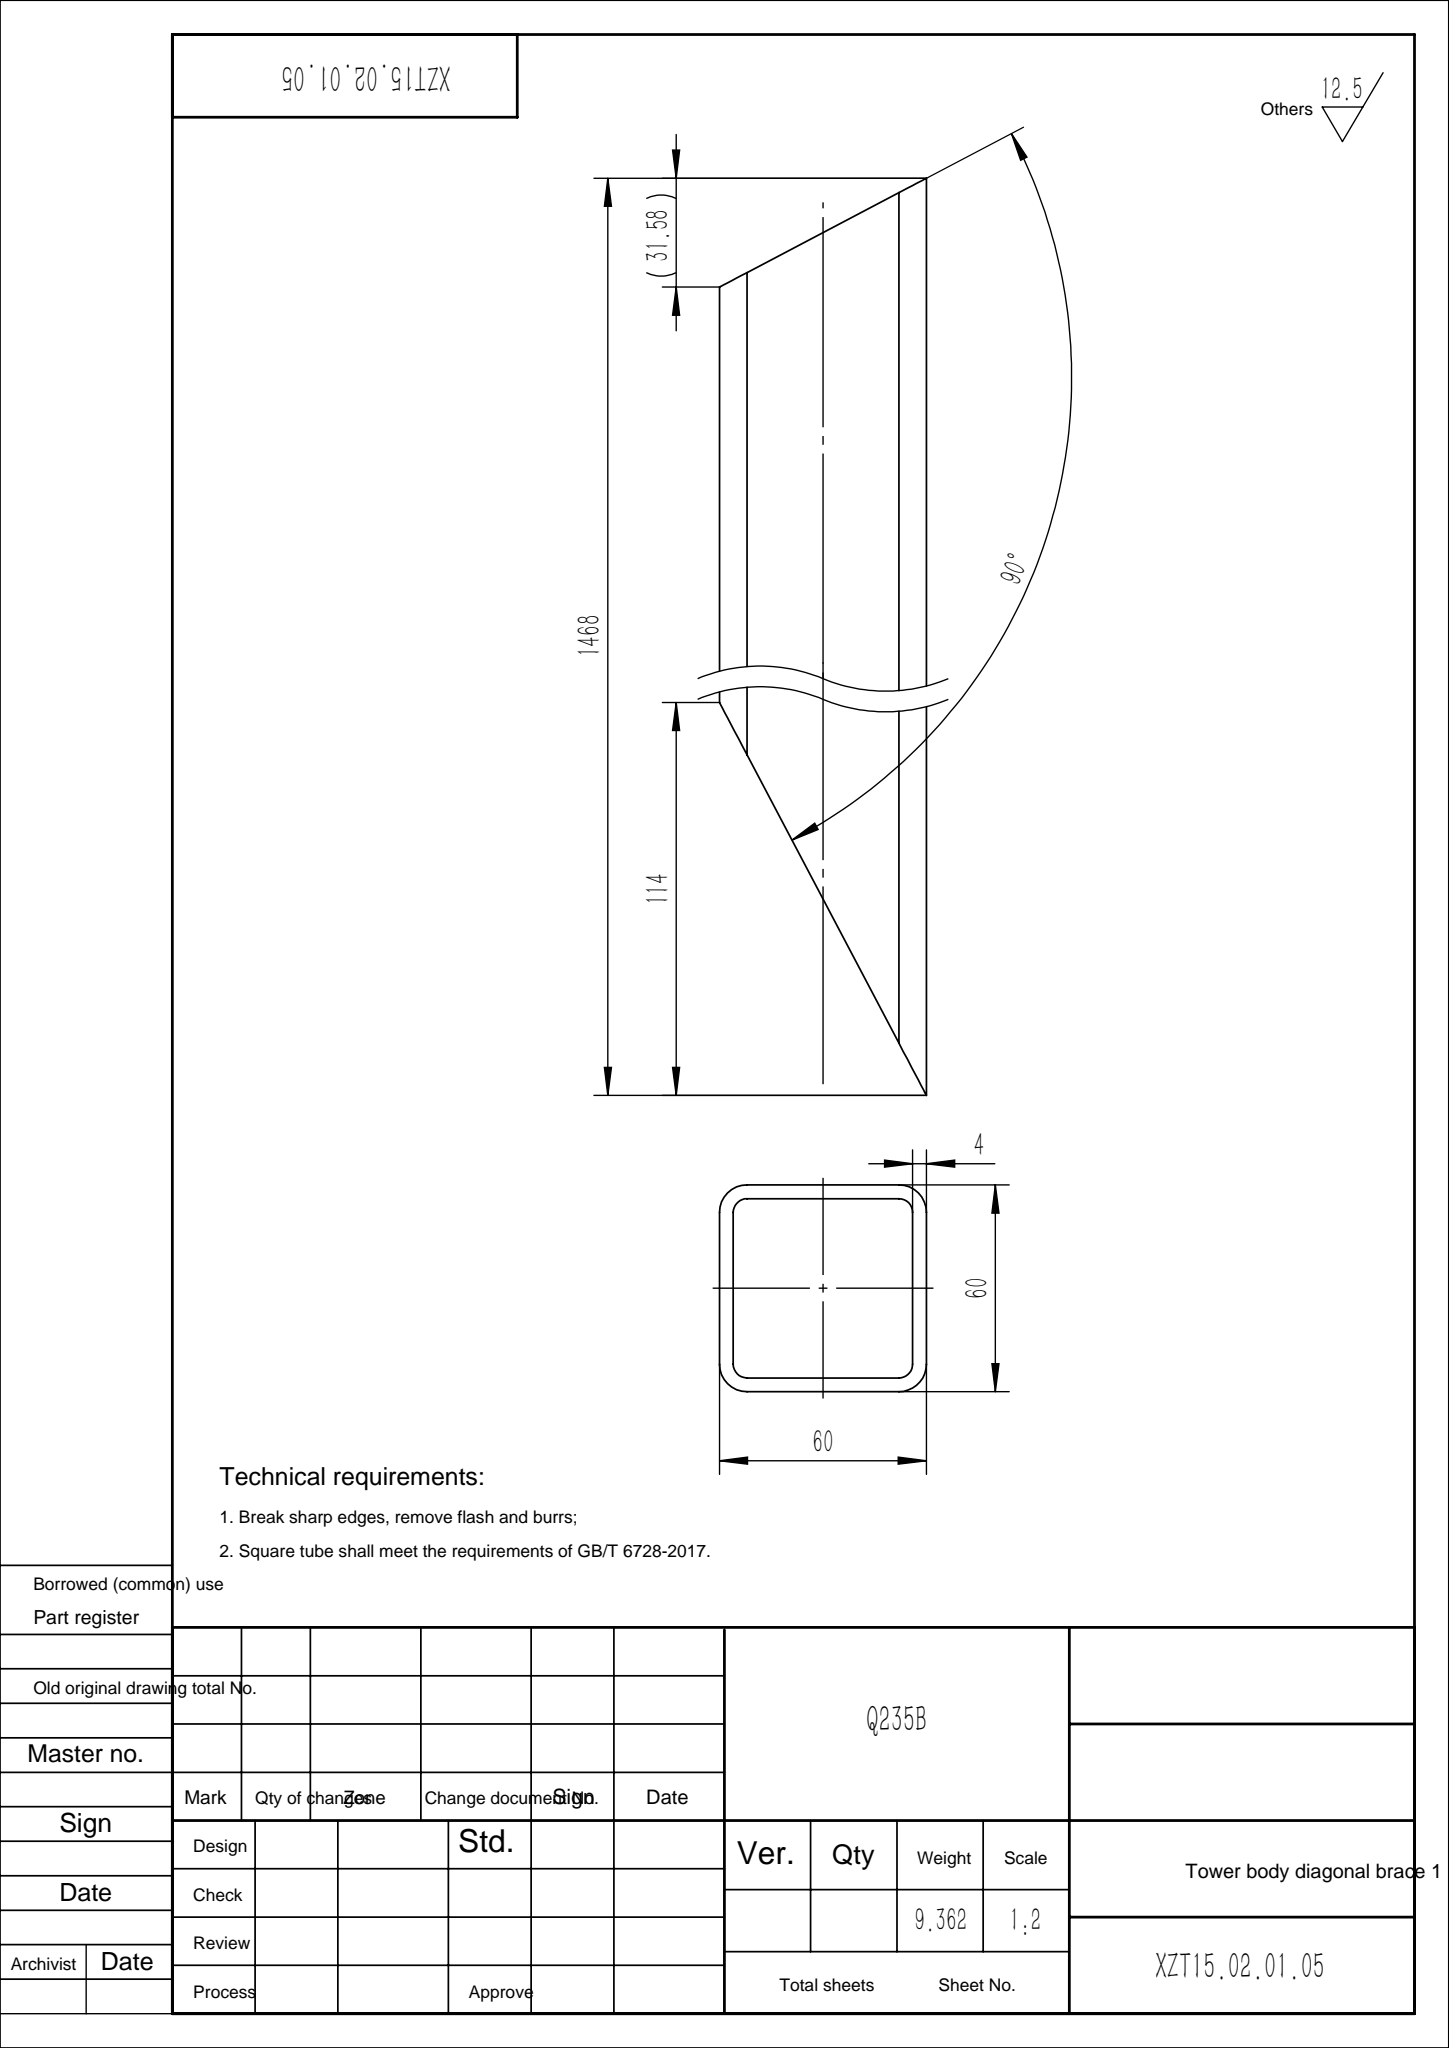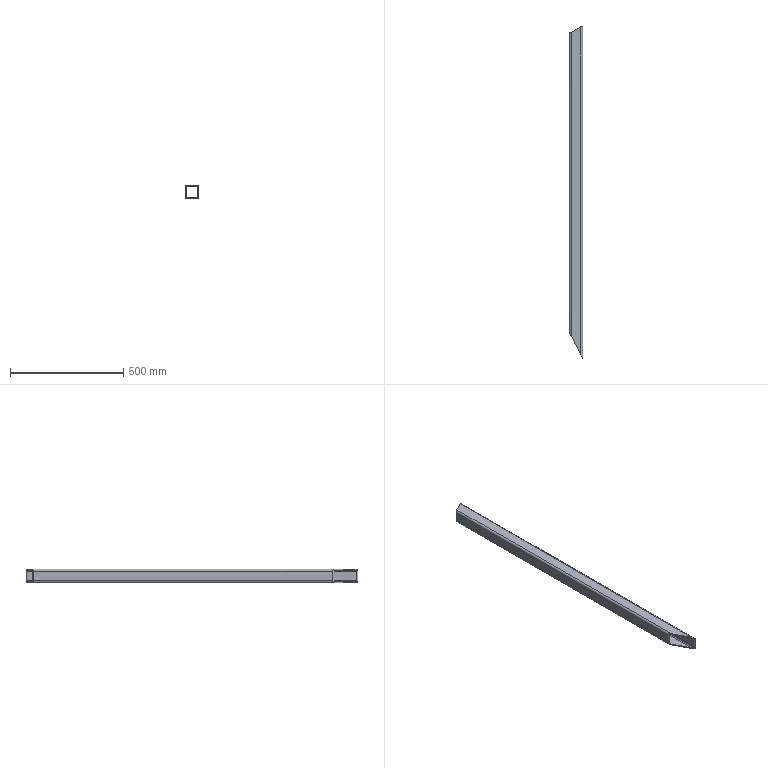Part | SolidWorks | features ICE 1, WeldMemberFeat 1, WeldmentFeature 1 | 1 solid | 18 faces | box 60 x 1468 x 60 mm | volume 1192621 mm3 | plane 10 | cylinder 8 | commonest cylinder face diameters 8 x4 16 x4
STEP:
#1=CARTESIAN_POINT('',(30.,0.,22.));
#2=VERTEX_POINT('',#1);
#3=CARTESIAN_POINT('',(30.,0.,-22.));
#4=VERTEX_POINT('',#3);
#5=CARTESIAN_POINT('',(30.,0.,-22.));
#6=DIRECTION('',(0.,0.,-1.));
#7=VECTOR('',#6,1000.);
#8=LINE('',#5,#7);
#9=EDGE_CURVE('',#2,#4,#8,.T.);
#10=ORIENTED_EDGE('',*,*,#9,.T.);
#11=CARTESIAN_POINT('',(30.,1468.,-22.));
#12=VERTEX_POINT('',#11);
#13=CARTESIAN_POINT('',(30.,1468.,-22.));
#14=DIRECTION('',(0.,-1.,0.));
#15=VECTOR('',#14,1000.);
#16=LINE('',#13,#15);
#17=EDGE_CURVE('',#12,#4,#16,.T.);
#18=ORIENTED_EDGE('',*,*,#17,.F.);
#19=CARTESIAN_POINT('',(30.,1468.,22.));
#20=VERTEX_POINT('',#19);
#21=CARTESIAN_POINT('',(30.,1468.,-22.));
#22=DIRECTION('',(0.,0.,-1.));
#23=VECTOR('',#22,1000.);
#24=LINE('',#21,#23);
#25=EDGE_CURVE('',#20,#12,#24,.T.);
#26=ORIENTED_EDGE('',*,*,#25,.F.);
#27=CARTESIAN_POINT('',(30.,1468.,22.));
#28=DIRECTION('',(0.,-1.,0.));
#29=VECTOR('',#28,1000.);
#30=LINE('',#27,#29);
#31=EDGE_CURVE('',#20,#2,#30,.T.);
#32=ORIENTED_EDGE('',*,*,#31,.T.);
#33=EDGE_LOOP('',(#10,#18,#26,#32));
#34=FACE_OUTER_BOUND('',#33,.T.);
#35=CARTESIAN_POINT('',(30.,1468.,-22.));
#36=DIRECTION('',(-1.,0.,0.));
#37=DIRECTION('',(0.,0.,1.));
#38=AXIS2_PLACEMENT_3D('',#35,#36,#37);
#39=PLANE('',#38);
#40=ADVANCED_FACE('',(#34),#39,.F.);
#41=CARTESIAN_POINT('',(-30.,1436.421,22.));
#42=VERTEX_POINT('',#41);
#43=CARTESIAN_POINT('',(-30.,114.,22.));
#44=VERTEX_POINT('',#43);
#45=CARTESIAN_POINT('',(-30.,1468.,22.));
#46=DIRECTION('',(0.,-1.,0.));
#47=VECTOR('',#46,1000.);
#48=LINE('',#45,#47);
#49=EDGE_CURVE('',#42,#44,#48,.T.);
#50=ORIENTED_EDGE('',*,*,#49,.F.);
#51=CARTESIAN_POINT('',(-30.,1436.421,-22.));
#52=VERTEX_POINT('',#51);
#53=CARTESIAN_POINT('',(-30.,1436.421,-30.));
#54=DIRECTION('',(0.,0.,1.));
#55=VECTOR('',#54,1000.);
#56=LINE('',#53,#55);
#57=EDGE_CURVE('',#52,#42,#56,.T.);
#58=ORIENTED_EDGE('',*,*,#57,.F.);
#59=CARTESIAN_POINT('',(-30.,114.,-22.));
#60=VERTEX_POINT('',#59);
#61=CARTESIAN_POINT('',(-30.,1468.,-22.));
#62=DIRECTION('',(0.,-1.,0.));
#63=VECTOR('',#62,1000.);
#64=LINE('',#61,#63);
#65=EDGE_CURVE('',#52,#60,#64,.T.);
#66=ORIENTED_EDGE('',*,*,#65,.T.);
#67=CARTESIAN_POINT('',(-30.,114.,-30.));
#68=DIRECTION('',(0.,0.,1.));
#69=VECTOR('',#68,1000.);
#70=LINE('',#67,#69);
#71=EDGE_CURVE('',#60,#44,#70,.T.);
#72=ORIENTED_EDGE('',*,*,#71,.T.);
#73=EDGE_LOOP('',(#50,#58,#66,#72));
#74=FACE_OUTER_BOUND('',#73,.T.);
#75=CARTESIAN_POINT('',(-30.,1468.,22.));
#76=DIRECTION('',(1.,0.,0.));
#77=DIRECTION('',(0.,0.,-1.));
#78=AXIS2_PLACEMENT_3D('',#75,#76,#77);
#79=PLANE('',#78);
#80=ADVANCED_FACE('',(#74),#79,.F.);
#81=ORIENTED_EDGE('',*,*,#65,.F.);
#82=CARTESIAN_POINT('',(-22.,1440.632,-30.));
#83=VERTEX_POINT('',#82);
#84=CARTESIAN_POINT('',(-30.,1436.421,-22.));
#85=CARTESIAN_POINT('',(-30.,1436.421,-26.686));
#86=CARTESIAN_POINT('',(-26.686,1438.165,-30.));
#87=CARTESIAN_POINT('',(-22.,1440.632,-30.));
#88=(BOUNDED_CURVE()B_SPLINE_CURVE(3,(#84,#85,#86,#87),.UNSPECIFIED.,.F.,.F.)B_SPLINE_CURVE_WITH_KNOTS((4,4),(0.,1.571),.UNSPECIFIED.)CURVE()GEOMETRIC_REPRESENTATION_ITEM()RATIONAL_B_SPLINE_CURVE((1.,0.8047,0.8047,1.))REPRESENTATION_ITEM(''));
#89=EDGE_CURVE('',#52,#83,#88,.T.);
#90=ORIENTED_EDGE('',*,*,#89,.T.);
#91=CARTESIAN_POINT('',(-22.,98.8,-30.));
#92=VERTEX_POINT('',#91);
#93=CARTESIAN_POINT('',(-22.,1468.,-30.));
#94=DIRECTION('',(0.,-1.,0.));
#95=VECTOR('',#94,1000.);
#96=LINE('',#93,#95);
#97=EDGE_CURVE('',#83,#92,#96,.T.);
#98=ORIENTED_EDGE('',*,*,#97,.T.);
#99=CARTESIAN_POINT('',(-22.,98.8,-30.));
#100=CARTESIAN_POINT('',(-26.686,107.704,-30.));
#101=CARTESIAN_POINT('',(-30.,114.,-26.686));
#102=CARTESIAN_POINT('',(-30.,114.,-22.));
#103=(BOUNDED_CURVE()B_SPLINE_CURVE(3,(#99,#100,#101,#102),.UNSPECIFIED.,.F.,.F.)B_SPLINE_CURVE_WITH_KNOTS((4,4),(1.571,3.142),.UNSPECIFIED.)CURVE()GEOMETRIC_REPRESENTATION_ITEM()RATIONAL_B_SPLINE_CURVE((1.,0.8047,0.8047,1.))REPRESENTATION_ITEM(''));
#104=EDGE_CURVE('',#92,#60,#103,.T.);
#105=ORIENTED_EDGE('',*,*,#104,.T.);
#106=EDGE_LOOP('',(#81,#90,#98,#105));
#107=FACE_OUTER_BOUND('',#106,.T.);
#108=CARTESIAN_POINT('',(-22.,1468.,-22.));
#109=DIRECTION('',(0.,-1.,0.));
#110=DIRECTION('',(0.,0.,-1.));
#111=AXIS2_PLACEMENT_3D('',#108,#109,#110);
#112=CYLINDRICAL_SURFACE('',#111,8.);
#113=ADVANCED_FACE('',(#107),#112,.T.);
#114=ORIENTED_EDGE('',*,*,#97,.F.);
#115=CARTESIAN_POINT('',(22.,1463.789,-30.));
#116=VERTEX_POINT('',#115);
#117=CARTESIAN_POINT('',(-30.,1436.421,-30.));
#118=DIRECTION('',(0.8849,0.4657,0.));
#119=VECTOR('',#118,1000.);
#120=LINE('',#117,#119);
#121=EDGE_CURVE('',#83,#116,#120,.T.);
#122=ORIENTED_EDGE('',*,*,#121,.T.);
#123=CARTESIAN_POINT('',(22.,15.2,-30.));
#124=VERTEX_POINT('',#123);
#125=CARTESIAN_POINT('',(22.,1468.,-30.));
#126=DIRECTION('',(0.,-1.,0.));
#127=VECTOR('',#126,1000.);
#128=LINE('',#125,#127);
#129=EDGE_CURVE('',#116,#124,#128,.T.);
#130=ORIENTED_EDGE('',*,*,#129,.T.);
#131=CARTESIAN_POINT('',(-30.,114.,-30.));
#132=DIRECTION('',(-0.4657,0.8849,0.));
#133=VECTOR('',#132,1000.);
#134=LINE('',#131,#133);
#135=EDGE_CURVE('',#124,#92,#134,.T.);
#136=ORIENTED_EDGE('',*,*,#135,.T.);
#137=EDGE_LOOP('',(#114,#122,#130,#136));
#138=FACE_OUTER_BOUND('',#137,.T.);
#139=CARTESIAN_POINT('',(22.,1468.,-30.));
#140=DIRECTION('',(0.,0.,1.));
#141=DIRECTION('',(1.,0.,0.));
#142=AXIS2_PLACEMENT_3D('',#139,#140,#141);
#143=PLANE('',#142);
#144=ADVANCED_FACE('',(#138),#143,.F.);
#145=ORIENTED_EDGE('',*,*,#129,.F.);
#146=CARTESIAN_POINT('',(22.,1463.789,-30.));
#147=CARTESIAN_POINT('',(26.686,1466.256,-30.));
#148=CARTESIAN_POINT('',(30.,1468.,-26.686));
#149=CARTESIAN_POINT('',(30.,1468.,-22.));
#150=(BOUNDED_CURVE()B_SPLINE_CURVE(3,(#146,#147,#148,#149),.UNSPECIFIED.,.F.,.T.)B_SPLINE_CURVE_WITH_KNOTS((4,4),(1.571,3.142),.UNSPECIFIED.)CURVE()GEOMETRIC_REPRESENTATION_ITEM()RATIONAL_B_SPLINE_CURVE((1.,0.8047,0.8047,1.))REPRESENTATION_ITEM(''));
#151=EDGE_CURVE('',#116,#12,#150,.T.);
#152=ORIENTED_EDGE('',*,*,#151,.T.);
#153=ORIENTED_EDGE('',*,*,#17,.T.);
#154=CARTESIAN_POINT('',(30.,0.,-22.));
#155=CARTESIAN_POINT('',(30.,0.,-26.686));
#156=CARTESIAN_POINT('',(26.686,6.296,-30.));
#157=CARTESIAN_POINT('',(22.,15.2,-30.));
#158=(BOUNDED_CURVE()B_SPLINE_CURVE(3,(#154,#155,#156,#157),.UNSPECIFIED.,.F.,.F.)B_SPLINE_CURVE_WITH_KNOTS((4,4),(0.,1.571),.UNSPECIFIED.)CURVE()GEOMETRIC_REPRESENTATION_ITEM()RATIONAL_B_SPLINE_CURVE((1.,0.8047,0.8047,1.))REPRESENTATION_ITEM(''));
#159=EDGE_CURVE('',#4,#124,#158,.T.);
#160=ORIENTED_EDGE('',*,*,#159,.T.);
#161=EDGE_LOOP('',(#145,#152,#153,#160));
#162=FACE_OUTER_BOUND('',#161,.T.);
#163=CARTESIAN_POINT('',(22.,1468.,-22.));
#164=DIRECTION('',(0.,-1.,0.));
#165=DIRECTION('',(0.,0.,-1.));
#166=AXIS2_PLACEMENT_3D('',#163,#164,#165);
#167=CYLINDRICAL_SURFACE('',#166,8.);
#168=ADVANCED_FACE('',(#162),#167,.T.);
#169=ORIENTED_EDGE('',*,*,#31,.F.);
#170=CARTESIAN_POINT('',(22.,1463.789,30.));
#171=VERTEX_POINT('',#170);
#172=CARTESIAN_POINT('',(30.,1468.,22.));
#173=CARTESIAN_POINT('',(30.,1468.,26.686));
#174=CARTESIAN_POINT('',(26.686,1466.256,30.));
#175=CARTESIAN_POINT('',(22.,1463.789,30.));
#176=(BOUNDED_CURVE()B_SPLINE_CURVE(3,(#172,#173,#174,#175),.UNSPECIFIED.,.F.,.F.)B_SPLINE_CURVE_WITH_KNOTS((4,4),(3.142,4.712),.UNSPECIFIED.)CURVE()GEOMETRIC_REPRESENTATION_ITEM()RATIONAL_B_SPLINE_CURVE((1.,0.8047,0.8047,1.))REPRESENTATION_ITEM(''));
#177=EDGE_CURVE('',#20,#171,#176,.T.);
#178=ORIENTED_EDGE('',*,*,#177,.T.);
#179=CARTESIAN_POINT('',(22.,15.2,30.));
#180=VERTEX_POINT('',#179);
#181=CARTESIAN_POINT('',(22.,1468.,30.));
#182=DIRECTION('',(0.,-1.,0.));
#183=VECTOR('',#182,1000.);
#184=LINE('',#181,#183);
#185=EDGE_CURVE('',#171,#180,#184,.T.);
#186=ORIENTED_EDGE('',*,*,#185,.T.);
#187=CARTESIAN_POINT('',(22.,15.2,30.));
#188=CARTESIAN_POINT('',(26.686,6.296,30.));
#189=CARTESIAN_POINT('',(30.,0.,26.686));
#190=CARTESIAN_POINT('',(30.,0.,22.));
#191=(BOUNDED_CURVE()B_SPLINE_CURVE(3,(#187,#188,#189,#190),.UNSPECIFIED.,.F.,.F.)B_SPLINE_CURVE_WITH_KNOTS((4,4),(4.712,6.283),.UNSPECIFIED.)CURVE()GEOMETRIC_REPRESENTATION_ITEM()RATIONAL_B_SPLINE_CURVE((1.,0.8047,0.8047,1.))REPRESENTATION_ITEM(''));
#192=EDGE_CURVE('',#180,#2,#191,.T.);
#193=ORIENTED_EDGE('',*,*,#192,.T.);
#194=EDGE_LOOP('',(#169,#178,#186,#193));
#195=FACE_OUTER_BOUND('',#194,.T.);
#196=CARTESIAN_POINT('',(22.,1468.,22.));
#197=DIRECTION('',(0.,-1.,0.));
#198=DIRECTION('',(0.,0.,-1.));
#199=AXIS2_PLACEMENT_3D('',#196,#197,#198);
#200=CYLINDRICAL_SURFACE('',#199,8.);
#201=ADVANCED_FACE('',(#195),#200,.T.);
#202=ORIENTED_EDGE('',*,*,#185,.F.);
#203=CARTESIAN_POINT('',(-22.,1440.632,30.));
#204=VERTEX_POINT('',#203);
#205=CARTESIAN_POINT('',(-10.72,1446.568,30.));
#206=DIRECTION('',(-0.8849,-0.4657,0.));
#207=VECTOR('',#206,1000.);
#208=LINE('',#205,#207);
#209=EDGE_CURVE('',#171,#204,#208,.T.);
#210=ORIENTED_EDGE('',*,*,#209,.T.);
#211=CARTESIAN_POINT('',(-22.,98.8,30.));
#212=VERTEX_POINT('',#211);
#213=CARTESIAN_POINT('',(-22.,1468.,30.));
#214=DIRECTION('',(0.,-1.,0.));
#215=VECTOR('',#214,1000.);
#216=LINE('',#213,#215);
#217=EDGE_CURVE('',#204,#212,#216,.T.);
#218=ORIENTED_EDGE('',*,*,#217,.T.);
#219=CARTESIAN_POINT('',(-586.312,1170.993,30.));
#220=DIRECTION('',(0.4657,-0.8849,0.));
#221=VECTOR('',#220,1000.);
#222=LINE('',#219,#221);
#223=EDGE_CURVE('',#212,#180,#222,.T.);
#224=ORIENTED_EDGE('',*,*,#223,.T.);
#225=EDGE_LOOP('',(#202,#210,#218,#224));
#226=FACE_OUTER_BOUND('',#225,.T.);
#227=CARTESIAN_POINT('',(-22.,1468.,30.));
#228=DIRECTION('',(0.,0.,-1.));
#229=DIRECTION('',(-1.,0.,0.));
#230=AXIS2_PLACEMENT_3D('',#227,#228,#229);
#231=PLANE('',#230);
#232=ADVANCED_FACE('',(#226),#231,.F.);
#233=ORIENTED_EDGE('',*,*,#217,.F.);
#234=CARTESIAN_POINT('',(-22.,1440.632,30.));
#235=CARTESIAN_POINT('',(-26.686,1438.165,30.));
#236=CARTESIAN_POINT('',(-30.,1436.421,26.686));
#237=CARTESIAN_POINT('',(-30.,1436.421,22.));
#238=(BOUNDED_CURVE()B_SPLINE_CURVE(3,(#234,#235,#236,#237),.UNSPECIFIED.,.F.,.F.)B_SPLINE_CURVE_WITH_KNOTS((4,4),(4.712,6.283),.UNSPECIFIED.)CURVE()GEOMETRIC_REPRESENTATION_ITEM()RATIONAL_B_SPLINE_CURVE((1.,0.8047,0.8047,1.))REPRESENTATION_ITEM(''));
#239=EDGE_CURVE('',#204,#42,#238,.T.);
#240=ORIENTED_EDGE('',*,*,#239,.T.);
#241=ORIENTED_EDGE('',*,*,#49,.T.);
#242=CARTESIAN_POINT('',(-30.,114.,22.));
#243=CARTESIAN_POINT('',(-30.,114.,26.686));
#244=CARTESIAN_POINT('',(-26.686,107.704,30.));
#245=CARTESIAN_POINT('',(-22.,98.8,30.));
#246=(BOUNDED_CURVE()B_SPLINE_CURVE(3,(#242,#243,#244,#245),.UNSPECIFIED.,.F.,.F.)B_SPLINE_CURVE_WITH_KNOTS((4,4),(3.142,4.712),.UNSPECIFIED.)CURVE()GEOMETRIC_REPRESENTATION_ITEM()RATIONAL_B_SPLINE_CURVE((1.,0.8047,0.8047,1.))REPRESENTATION_ITEM(''));
#247=EDGE_CURVE('',#44,#212,#246,.T.);
#248=ORIENTED_EDGE('',*,*,#247,.T.);
#249=EDGE_LOOP('',(#233,#240,#241,#248));
#250=FACE_OUTER_BOUND('',#249,.T.);
#251=CARTESIAN_POINT('',(-22.,1468.,22.));
#252=DIRECTION('',(0.,-1.,0.));
#253=DIRECTION('',(0.,0.,-1.));
#254=AXIS2_PLACEMENT_3D('',#251,#252,#253);
#255=CYLINDRICAL_SURFACE('',#254,8.);
#256=ADVANCED_FACE('',(#250),#255,.T.);
#257=CARTESIAN_POINT('',(22.,15.2,26.));
#258=VERTEX_POINT('',#257);
#259=CARTESIAN_POINT('',(26.,7.6,22.));
#260=VERTEX_POINT('',#259);
#261=CARTESIAN_POINT('',(22.,15.2,26.));
#262=CARTESIAN_POINT('',(24.343,10.748,26.));
#263=CARTESIAN_POINT('',(26.,7.6,24.343));
#264=CARTESIAN_POINT('',(26.,7.6,22.));
#265=(BOUNDED_CURVE()B_SPLINE_CURVE(3,(#261,#262,#263,#264),.UNSPECIFIED.,.F.,.F.)B_SPLINE_CURVE_WITH_KNOTS((4,4),(4.712,6.283),.UNSPECIFIED.)CURVE()GEOMETRIC_REPRESENTATION_ITEM()RATIONAL_B_SPLINE_CURVE((1.,0.8047,0.8047,1.))REPRESENTATION_ITEM(''));
#266=EDGE_CURVE('',#258,#260,#265,.T.);
#267=ORIENTED_EDGE('',*,*,#266,.T.);
#268=CARTESIAN_POINT('',(26.,7.6,-22.));
#269=VERTEX_POINT('',#268);
#270=CARTESIAN_POINT('',(26.,7.6,-22.));
#271=DIRECTION('',(0.,0.,-1.));
#272=VECTOR('',#271,1000.);
#273=LINE('',#270,#272);
#274=EDGE_CURVE('',#260,#269,#273,.T.);
#275=ORIENTED_EDGE('',*,*,#274,.T.);
#276=CARTESIAN_POINT('',(22.,15.2,-26.));
#277=VERTEX_POINT('',#276);
#278=CARTESIAN_POINT('',(26.,7.6,-22.));
#279=CARTESIAN_POINT('',(26.,7.6,-24.343));
#280=CARTESIAN_POINT('',(24.343,10.748,-26.));
#281=CARTESIAN_POINT('',(22.,15.2,-26.));
#282=(BOUNDED_CURVE()B_SPLINE_CURVE(3,(#278,#279,#280,#281),.UNSPECIFIED.,.F.,.F.)B_SPLINE_CURVE_WITH_KNOTS((4,4),(0.,1.571),.UNSPECIFIED.)CURVE()GEOMETRIC_REPRESENTATION_ITEM()RATIONAL_B_SPLINE_CURVE((1.,0.8047,0.8047,1.))REPRESENTATION_ITEM(''));
#283=EDGE_CURVE('',#269,#277,#282,.T.);
#284=ORIENTED_EDGE('',*,*,#283,.T.);
#285=CARTESIAN_POINT('',(-22.,98.8,-26.));
#286=VERTEX_POINT('',#285);
#287=CARTESIAN_POINT('',(-576.768,1152.859,-26.));
#288=DIRECTION('',(-0.4657,0.8849,0.));
#289=VECTOR('',#288,1000.);
#290=LINE('',#287,#289);
#291=EDGE_CURVE('',#277,#286,#290,.T.);
#292=ORIENTED_EDGE('',*,*,#291,.T.);
#293=CARTESIAN_POINT('',(-26.,106.4,-22.));
#294=VERTEX_POINT('',#293);
#295=CARTESIAN_POINT('',(-22.,98.8,-26.));
#296=CARTESIAN_POINT('',(-24.343,103.252,-26.));
#297=CARTESIAN_POINT('',(-26.,106.4,-24.343));
#298=CARTESIAN_POINT('',(-26.,106.4,-22.));
#299=(BOUNDED_CURVE()B_SPLINE_CURVE(3,(#295,#296,#297,#298),.UNSPECIFIED.,.F.,.T.)B_SPLINE_CURVE_WITH_KNOTS((4,4),(1.571,3.142),.UNSPECIFIED.)CURVE()GEOMETRIC_REPRESENTATION_ITEM()RATIONAL_B_SPLINE_CURVE((1.,0.8047,0.8047,1.))REPRESENTATION_ITEM(''));
#300=EDGE_CURVE('',#286,#294,#299,.T.);
#301=ORIENTED_EDGE('',*,*,#300,.T.);
#302=CARTESIAN_POINT('',(-26.,106.4,22.));
#303=VERTEX_POINT('',#302);
#304=CARTESIAN_POINT('',(-26.,106.4,22.));
#305=DIRECTION('',(0.,0.,1.));
#306=VECTOR('',#305,1000.);
#307=LINE('',#304,#306);
#308=EDGE_CURVE('',#294,#303,#307,.T.);
#309=ORIENTED_EDGE('',*,*,#308,.T.);
#310=CARTESIAN_POINT('',(-22.,98.8,26.));
#311=VERTEX_POINT('',#310);
#312=CARTESIAN_POINT('',(-26.,106.4,22.));
#313=CARTESIAN_POINT('',(-26.,106.4,24.343));
#314=CARTESIAN_POINT('',(-24.343,103.252,26.));
#315=CARTESIAN_POINT('',(-22.,98.8,26.));
#316=(BOUNDED_CURVE()B_SPLINE_CURVE(3,(#312,#313,#314,#315),.UNSPECIFIED.,.F.,.F.)B_SPLINE_CURVE_WITH_KNOTS((4,4),(3.142,4.712),.UNSPECIFIED.)CURVE()GEOMETRIC_REPRESENTATION_ITEM()RATIONAL_B_SPLINE_CURVE((1.,0.8047,0.8047,1.))REPRESENTATION_ITEM(''));
#317=EDGE_CURVE('',#303,#311,#316,.T.);
#318=ORIENTED_EDGE('',*,*,#317,.T.);
#319=CARTESIAN_POINT('',(-586.312,1170.993,26.));
#320=DIRECTION('',(0.4657,-0.8849,0.));
#321=VECTOR('',#320,1000.);
#322=LINE('',#319,#321);
#323=EDGE_CURVE('',#311,#258,#322,.T.);
#324=ORIENTED_EDGE('',*,*,#323,.T.);
#325=EDGE_LOOP('',(#267,#275,#284,#292,#301,#309,#318,#324));
#326=FACE_BOUND('',#325,.T.);
#327=ORIENTED_EDGE('',*,*,#71,.F.);
#328=ORIENTED_EDGE('',*,*,#104,.F.);
#329=ORIENTED_EDGE('',*,*,#135,.F.);
#330=ORIENTED_EDGE('',*,*,#159,.F.);
#331=ORIENTED_EDGE('',*,*,#9,.F.);
#332=ORIENTED_EDGE('',*,*,#192,.F.);
#333=ORIENTED_EDGE('',*,*,#223,.F.);
#334=ORIENTED_EDGE('',*,*,#247,.F.);
#335=EDGE_LOOP('',(#327,#328,#329,#330,#331,#332,#333,#334));
#336=FACE_OUTER_BOUND('',#335,.T.);
#337=CARTESIAN_POINT('',(-30.,114.,-30.));
#338=DIRECTION('',(0.8849,0.4657,0.));
#339=DIRECTION('',(-0.4657,0.8849,0.));
#340=AXIS2_PLACEMENT_3D('',#337,#338,#339);
#341=PLANE('',#340);
#342=ADVANCED_FACE('',(#326,#336),#341,.F.);
#343=CARTESIAN_POINT('',(26.,1465.895,22.));
#344=VERTEX_POINT('',#343);
#345=CARTESIAN_POINT('',(22.,1463.789,26.));
#346=VERTEX_POINT('',#345);
#347=CARTESIAN_POINT('',(26.,1465.895,22.));
#348=CARTESIAN_POINT('',(26.,1465.895,24.343));
#349=CARTESIAN_POINT('',(24.343,1465.023,26.));
#350=CARTESIAN_POINT('',(22.,1463.789,26.));
#351=(BOUNDED_CURVE()B_SPLINE_CURVE(3,(#347,#348,#349,#350),.UNSPECIFIED.,.F.,.F.)B_SPLINE_CURVE_WITH_KNOTS((4,4),(3.142,4.712),.UNSPECIFIED.)CURVE()GEOMETRIC_REPRESENTATION_ITEM()RATIONAL_B_SPLINE_CURVE((1.,0.8047,0.8047,1.))REPRESENTATION_ITEM(''));
#352=EDGE_CURVE('',#344,#346,#351,.T.);
#353=ORIENTED_EDGE('',*,*,#352,.T.);
#354=CARTESIAN_POINT('',(-22.,1440.632,26.));
#355=VERTEX_POINT('',#354);
#356=CARTESIAN_POINT('',(-10.72,1446.568,26.));
#357=DIRECTION('',(-0.8849,-0.4657,0.));
#358=VECTOR('',#357,1000.);
#359=LINE('',#356,#358);
#360=EDGE_CURVE('',#346,#355,#359,.T.);
#361=ORIENTED_EDGE('',*,*,#360,.T.);
#362=CARTESIAN_POINT('',(-26.,1438.526,22.));
#363=VERTEX_POINT('',#362);
#364=CARTESIAN_POINT('',(-22.,1440.632,26.));
#365=CARTESIAN_POINT('',(-24.343,1439.398,26.));
#366=CARTESIAN_POINT('',(-26.,1438.526,24.343));
#367=CARTESIAN_POINT('',(-26.,1438.526,22.));
#368=(BOUNDED_CURVE()B_SPLINE_CURVE(3,(#364,#365,#366,#367),.UNSPECIFIED.,.F.,.F.)B_SPLINE_CURVE_WITH_KNOTS((4,4),(4.712,6.283),.UNSPECIFIED.)CURVE()GEOMETRIC_REPRESENTATION_ITEM()RATIONAL_B_SPLINE_CURVE((1.,0.8047,0.8047,1.))REPRESENTATION_ITEM(''));
#369=EDGE_CURVE('',#355,#363,#368,.T.);
#370=ORIENTED_EDGE('',*,*,#369,.T.);
#371=CARTESIAN_POINT('',(-26.,1438.526,-22.));
#372=VERTEX_POINT('',#371);
#373=CARTESIAN_POINT('',(-26.,1438.526,22.));
#374=DIRECTION('',(0.,0.,-1.));
#375=VECTOR('',#374,1000.);
#376=LINE('',#373,#375);
#377=EDGE_CURVE('',#363,#372,#376,.T.);
#378=ORIENTED_EDGE('',*,*,#377,.T.);
#379=CARTESIAN_POINT('',(-22.,1440.632,-26.));
#380=VERTEX_POINT('',#379);
#381=CARTESIAN_POINT('',(-26.,1438.526,-22.));
#382=CARTESIAN_POINT('',(-26.,1438.526,-24.343));
#383=CARTESIAN_POINT('',(-24.343,1439.398,-26.));
#384=CARTESIAN_POINT('',(-22.,1440.632,-26.));
#385=(BOUNDED_CURVE()B_SPLINE_CURVE(3,(#381,#382,#383,#384),.UNSPECIFIED.,.F.,.F.)B_SPLINE_CURVE_WITH_KNOTS((4,4),(0.,1.571),.UNSPECIFIED.)CURVE()GEOMETRIC_REPRESENTATION_ITEM()RATIONAL_B_SPLINE_CURVE((1.,0.8047,0.8047,1.))REPRESENTATION_ITEM(''));
#386=EDGE_CURVE('',#372,#380,#385,.T.);
#387=ORIENTED_EDGE('',*,*,#386,.T.);
#388=CARTESIAN_POINT('',(22.,1463.789,-26.));
#389=VERTEX_POINT('',#388);
#390=CARTESIAN_POINT('',(23.735,1464.703,-26.));
#391=DIRECTION('',(0.8849,0.4657,0.));
#392=VECTOR('',#391,1000.);
#393=LINE('',#390,#392);
#394=EDGE_CURVE('',#380,#389,#393,.T.);
#395=ORIENTED_EDGE('',*,*,#394,.T.);
#396=CARTESIAN_POINT('',(26.,1465.895,-22.));
#397=VERTEX_POINT('',#396);
#398=CARTESIAN_POINT('',(22.,1463.789,-26.));
#399=CARTESIAN_POINT('',(24.343,1465.023,-26.));
#400=CARTESIAN_POINT('',(26.,1465.895,-24.343));
#401=CARTESIAN_POINT('',(26.,1465.895,-22.));
#402=(BOUNDED_CURVE()B_SPLINE_CURVE(3,(#398,#399,#400,#401),.UNSPECIFIED.,.F.,.F.)B_SPLINE_CURVE_WITH_KNOTS((4,4),(1.571,3.142),.UNSPECIFIED.)CURVE()GEOMETRIC_REPRESENTATION_ITEM()RATIONAL_B_SPLINE_CURVE((1.,0.8047,0.8047,1.))REPRESENTATION_ITEM(''));
#403=EDGE_CURVE('',#389,#397,#402,.T.);
#404=ORIENTED_EDGE('',*,*,#403,.T.);
#405=CARTESIAN_POINT('',(26.,1465.895,-22.));
#406=DIRECTION('',(0.,0.,1.));
#407=VECTOR('',#406,1000.);
#408=LINE('',#405,#407);
#409=EDGE_CURVE('',#397,#344,#408,.T.);
#410=ORIENTED_EDGE('',*,*,#409,.T.);
#411=EDGE_LOOP('',(#353,#361,#370,#378,#387,#395,#404,#410));
#412=FACE_BOUND('',#411,.T.);
#413=ORIENTED_EDGE('',*,*,#209,.F.);
#414=ORIENTED_EDGE('',*,*,#177,.F.);
#415=ORIENTED_EDGE('',*,*,#25,.T.);
#416=ORIENTED_EDGE('',*,*,#151,.F.);
#417=ORIENTED_EDGE('',*,*,#121,.F.);
#418=ORIENTED_EDGE('',*,*,#89,.F.);
#419=ORIENTED_EDGE('',*,*,#57,.T.);
#420=ORIENTED_EDGE('',*,*,#239,.F.);
#421=EDGE_LOOP('',(#413,#414,#415,#416,#417,#418,#419,#420));
#422=FACE_OUTER_BOUND('',#421,.T.);
#423=CARTESIAN_POINT('',(-30.,1436.421,-30.));
#424=DIRECTION('',(0.4657,-0.8849,0.));
#425=DIRECTION('',(0.8849,0.4657,0.));
#426=AXIS2_PLACEMENT_3D('',#423,#424,#425);
#427=PLANE('',#426);
#428=ADVANCED_FACE('',(#412,#422),#427,.F.);
#429=ORIENTED_EDGE('',*,*,#352,.F.);
#430=CARTESIAN_POINT('',(26.,1468.,22.));
#431=DIRECTION('',(0.,-1.,0.));
#432=VECTOR('',#431,1000.);
#433=LINE('',#430,#432);
#434=EDGE_CURVE('',#344,#260,#433,.T.);
#435=ORIENTED_EDGE('',*,*,#434,.T.);
#436=ORIENTED_EDGE('',*,*,#266,.F.);
#437=CARTESIAN_POINT('',(22.,1468.,26.));
#438=DIRECTION('',(0.,-1.,0.));
#439=VECTOR('',#438,1000.);
#440=LINE('',#437,#439);
#441=EDGE_CURVE('',#346,#258,#440,.T.);
#442=ORIENTED_EDGE('',*,*,#441,.F.);
#443=EDGE_LOOP('',(#429,#435,#436,#442));
#444=FACE_OUTER_BOUND('',#443,.T.);
#445=CARTESIAN_POINT('',(22.,1468.,22.));
#446=DIRECTION('',(0.,-1.,0.));
#447=DIRECTION('',(0.,0.,-1.));
#448=AXIS2_PLACEMENT_3D('',#445,#446,#447);
#449=CYLINDRICAL_SURFACE('',#448,4.);
#450=ADVANCED_FACE('',(#444),#449,.F.);
#451=ORIENTED_EDGE('',*,*,#360,.F.);
#452=ORIENTED_EDGE('',*,*,#441,.T.);
#453=ORIENTED_EDGE('',*,*,#323,.F.);
#454=CARTESIAN_POINT('',(-22.,1468.,26.));
#455=DIRECTION('',(0.,-1.,0.));
#456=VECTOR('',#455,1000.);
#457=LINE('',#454,#456);
#458=EDGE_CURVE('',#355,#311,#457,.T.);
#459=ORIENTED_EDGE('',*,*,#458,.F.);
#460=EDGE_LOOP('',(#451,#452,#453,#459));
#461=FACE_OUTER_BOUND('',#460,.T.);
#462=CARTESIAN_POINT('',(-22.,1468.,26.));
#463=DIRECTION('',(0.,0.,-1.));
#464=DIRECTION('',(-1.,0.,0.));
#465=AXIS2_PLACEMENT_3D('',#462,#463,#464);
#466=PLANE('',#465);
#467=ADVANCED_FACE('',(#461),#466,.T.);
#468=ORIENTED_EDGE('',*,*,#369,.F.);
#469=ORIENTED_EDGE('',*,*,#458,.T.);
#470=ORIENTED_EDGE('',*,*,#317,.F.);
#471=CARTESIAN_POINT('',(-26.,1468.,22.));
#472=DIRECTION('',(0.,-1.,0.));
#473=VECTOR('',#472,1000.);
#474=LINE('',#471,#473);
#475=EDGE_CURVE('',#363,#303,#474,.T.);
#476=ORIENTED_EDGE('',*,*,#475,.F.);
#477=EDGE_LOOP('',(#468,#469,#470,#476));
#478=FACE_OUTER_BOUND('',#477,.T.);
#479=CARTESIAN_POINT('',(-22.,1468.,22.));
#480=DIRECTION('',(0.,-1.,0.));
#481=DIRECTION('',(0.,0.,-1.));
#482=AXIS2_PLACEMENT_3D('',#479,#480,#481);
#483=CYLINDRICAL_SURFACE('',#482,4.);
#484=ADVANCED_FACE('',(#478),#483,.F.);
#485=ORIENTED_EDGE('',*,*,#377,.F.);
#486=ORIENTED_EDGE('',*,*,#475,.T.);
#487=ORIENTED_EDGE('',*,*,#308,.F.);
#488=CARTESIAN_POINT('',(-26.,1468.,-22.));
#489=DIRECTION('',(0.,-1.,0.));
#490=VECTOR('',#489,1000.);
#491=LINE('',#488,#490);
#492=EDGE_CURVE('',#372,#294,#491,.T.);
#493=ORIENTED_EDGE('',*,*,#492,.F.);
#494=EDGE_LOOP('',(#485,#486,#487,#493));
#495=FACE_OUTER_BOUND('',#494,.T.);
#496=CARTESIAN_POINT('',(-26.,1468.,22.));
#497=DIRECTION('',(1.,0.,0.));
#498=DIRECTION('',(0.,0.,-1.));
#499=AXIS2_PLACEMENT_3D('',#496,#497,#498);
#500=PLANE('',#499);
#501=ADVANCED_FACE('',(#495),#500,.T.);
#502=ORIENTED_EDGE('',*,*,#386,.F.);
#503=ORIENTED_EDGE('',*,*,#492,.T.);
#504=ORIENTED_EDGE('',*,*,#300,.F.);
#505=CARTESIAN_POINT('',(-22.,1468.,-26.));
#506=DIRECTION('',(0.,-1.,0.));
#507=VECTOR('',#506,1000.);
#508=LINE('',#505,#507);
#509=EDGE_CURVE('',#380,#286,#508,.T.);
#510=ORIENTED_EDGE('',*,*,#509,.F.);
#511=EDGE_LOOP('',(#502,#503,#504,#510));
#512=FACE_OUTER_BOUND('',#511,.T.);
#513=CARTESIAN_POINT('',(-22.,1468.,-22.));
#514=DIRECTION('',(0.,-1.,0.));
#515=DIRECTION('',(0.,0.,-1.));
#516=AXIS2_PLACEMENT_3D('',#513,#514,#515);
#517=CYLINDRICAL_SURFACE('',#516,4.);
#518=ADVANCED_FACE('',(#512),#517,.F.);
#519=ORIENTED_EDGE('',*,*,#394,.F.);
#520=ORIENTED_EDGE('',*,*,#509,.T.);
#521=ORIENTED_EDGE('',*,*,#291,.F.);
#522=CARTESIAN_POINT('',(22.,1468.,-26.));
#523=DIRECTION('',(0.,-1.,0.));
#524=VECTOR('',#523,1000.);
#525=LINE('',#522,#524);
#526=EDGE_CURVE('',#389,#277,#525,.T.);
#527=ORIENTED_EDGE('',*,*,#526,.F.);
#528=EDGE_LOOP('',(#519,#520,#521,#527));
#529=FACE_OUTER_BOUND('',#528,.T.);
#530=CARTESIAN_POINT('',(22.,1468.,-26.));
#531=DIRECTION('',(0.,0.,1.));
#532=DIRECTION('',(1.,0.,0.));
#533=AXIS2_PLACEMENT_3D('',#530,#531,#532);
#534=PLANE('',#533);
#535=ADVANCED_FACE('',(#529),#534,.T.);
#536=ORIENTED_EDGE('',*,*,#403,.F.);
#537=ORIENTED_EDGE('',*,*,#526,.T.);
#538=ORIENTED_EDGE('',*,*,#283,.F.);
#539=CARTESIAN_POINT('',(26.,1468.,-22.));
#540=DIRECTION('',(0.,-1.,0.));
#541=VECTOR('',#540,1000.);
#542=LINE('',#539,#541);
#543=EDGE_CURVE('',#397,#269,#542,.T.);
#544=ORIENTED_EDGE('',*,*,#543,.F.);
#545=EDGE_LOOP('',(#536,#537,#538,#544));
#546=FACE_OUTER_BOUND('',#545,.T.);
#547=CARTESIAN_POINT('',(22.,1468.,-22.));
#548=DIRECTION('',(0.,-1.,0.));
#549=DIRECTION('',(0.,0.,-1.));
#550=AXIS2_PLACEMENT_3D('',#547,#548,#549);
#551=CYLINDRICAL_SURFACE('',#550,4.);
#552=ADVANCED_FACE('',(#546),#551,.F.);
#553=ORIENTED_EDGE('',*,*,#409,.F.);
#554=ORIENTED_EDGE('',*,*,#543,.T.);
#555=ORIENTED_EDGE('',*,*,#274,.F.);
#556=ORIENTED_EDGE('',*,*,#434,.F.);
#557=EDGE_LOOP('',(#553,#554,#555,#556));
#558=FACE_OUTER_BOUND('',#557,.T.);
#559=CARTESIAN_POINT('',(26.,1468.,-22.));
#560=DIRECTION('',(-1.,0.,0.));
#561=DIRECTION('',(0.,0.,1.));
#562=AXIS2_PLACEMENT_3D('',#559,#560,#561);
#563=PLANE('',#562);
#564=ADVANCED_FACE('',(#558),#563,.T.);
#565=CLOSED_SHELL('',(#40,#80,#113,#144,#168,#201,#232,#256,#342,#428,#450,#467,#484,#501,#518,#535,#552,#564));
#566=MANIFOLD_SOLID_BREP('',#565);
#567=CARTESIAN_POINT('',(0.,0.,0.));
#568=DIRECTION('',(0.,0.,1.));
#569=DIRECTION('',(1.,0.,0.));
#570=AXIS2_PLACEMENT_3D('',#567,#568,#569);
#571=(LENGTH_UNIT()NAMED_UNIT(*)SI_UNIT(.MILLI.,.METRE.));
#572=UNCERTAINTY_MEASURE_WITH_UNIT(LENGTH_MEASURE(0.00001),#571,'','');
#573=(NAMED_UNIT(*)PLANE_ANGLE_UNIT()SI_UNIT($,.RADIAN.));
#574=(NAMED_UNIT(*)SI_UNIT($,.STERADIAN.)SOLID_ANGLE_UNIT());
#575=(GEOMETRIC_REPRESENTATION_CONTEXT(3)GLOBAL_UNCERTAINTY_ASSIGNED_CONTEXT((#572))GLOBAL_UNIT_ASSIGNED_CONTEXT((#571,#573,#574))REPRESENTATION_CONTEXT('',''));
#576=ADVANCED_BREP_SHAPE_REPRESENTATION('',(#566,#570),#575);